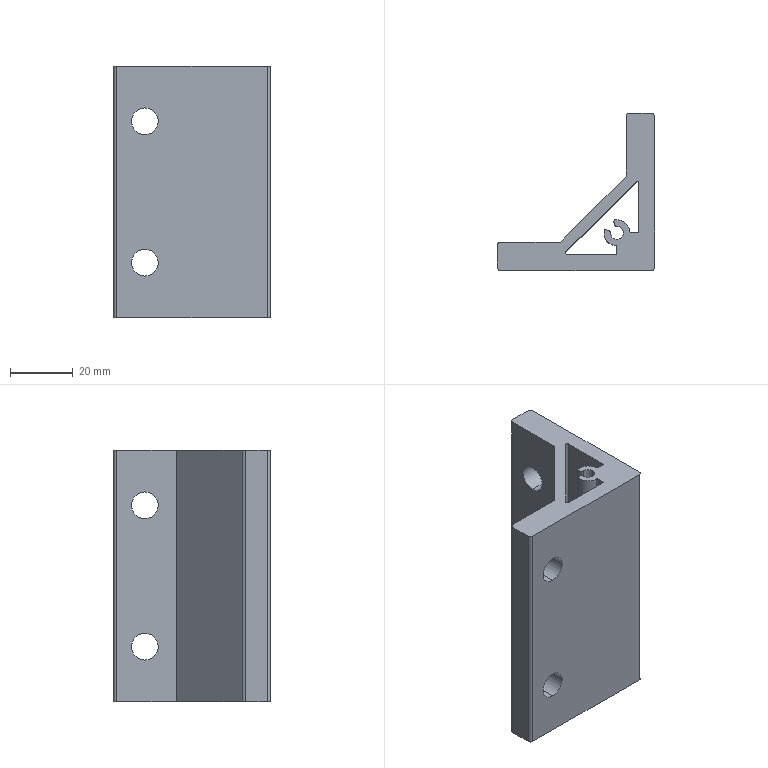Part | STEP file | 001-010-ABC01-4510-50-80 | 1 solid | 45 faces | box 50 x 50 x 80 mm | volume 63404 mm3 | cylinder 29 | plane 16 | commonest cylinder face diameters 1 x11 8.5 x8 2 x5 4.2 x3 8.2 x2